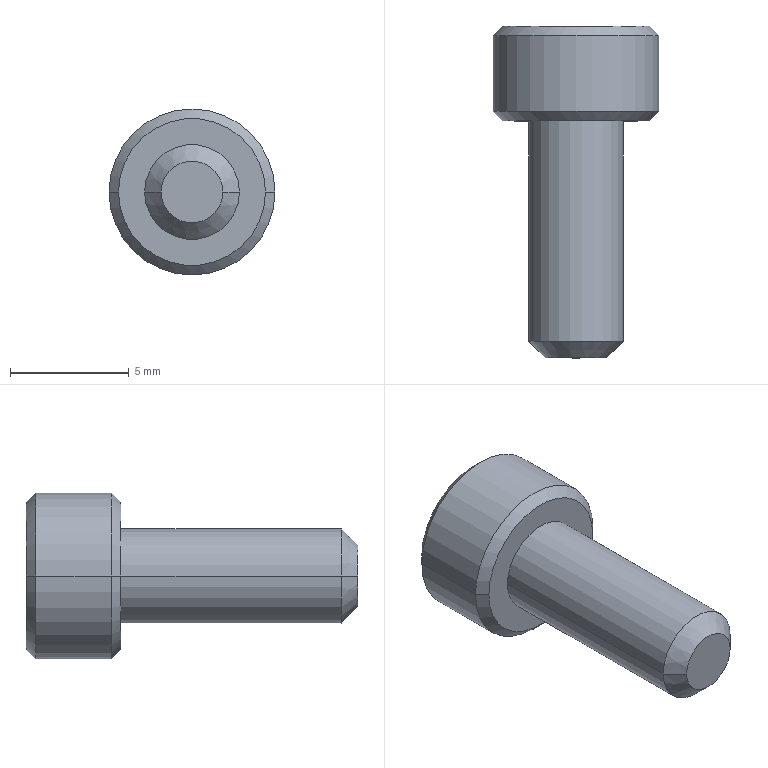Part | STEP file | BB62-M4-10L | 1 solid | 27 faces | box 7 x 14 x 7 mm | volume 255.049 mm3 | plane 15 | cone 8 | cylinder 4 | commonest cylinder face diameters 4 x2 7 x2